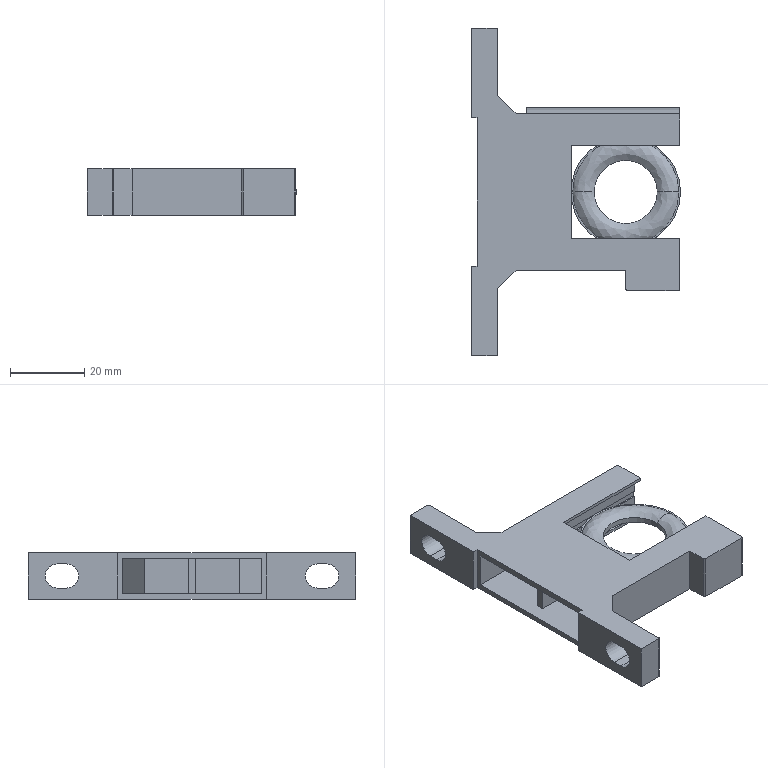Part | STEP file | Copy 1^GFC30015-A-F1 | 1 solid | 78 faces | box 56.25 x 88 x 12.5 mm | volume 17185 mm3 | plane 58 | cylinder 16 | spline 4 | commonest cylinder face diameters 4 x4 6.5 x4 0.6 x2 1 x2 17 x2 23.5 x1